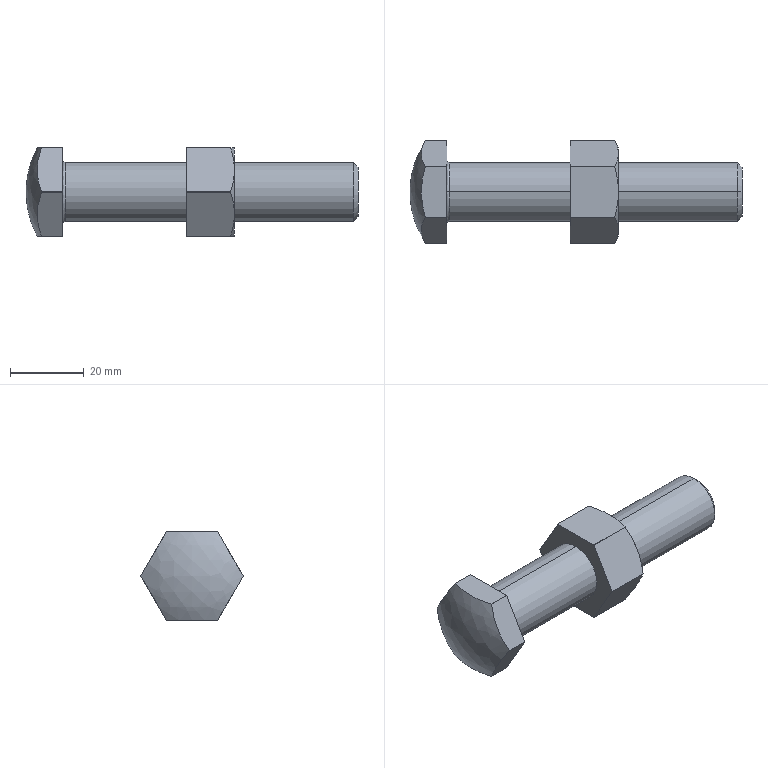Part | STEP file | STBB16-80-MISIMI | 2 solids | 47 faces | box 90 x 27.7 x 24 mm | volume 24665 mm3 | cylinder 16 | plane 16 | cone 12 | spline 3 | commonest cylinder face diameters 27.7 x12 13.835 x2 16 x2